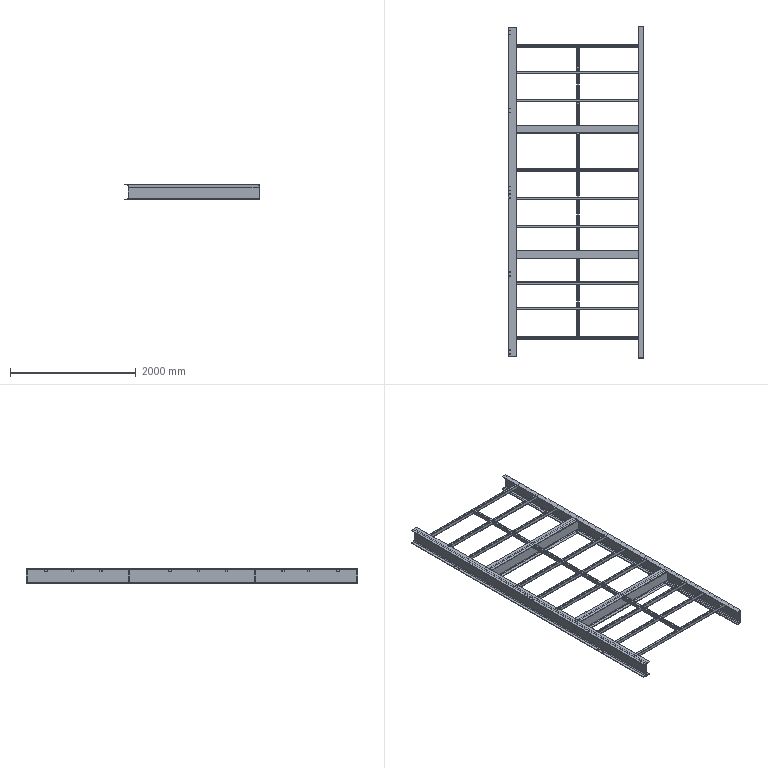Part | STEP file | PN_0040 second-floor platform deck_Default<As Machined> | 23 solids | 589 faces | box 2148 x 5275 x 250 mm | volume 68076276 mm3 | plane 357 | cylinder 232 | commonest cylinder face diameters 12 x100 6 x76 24 x24 6.8 x12 26 x12 18 x8